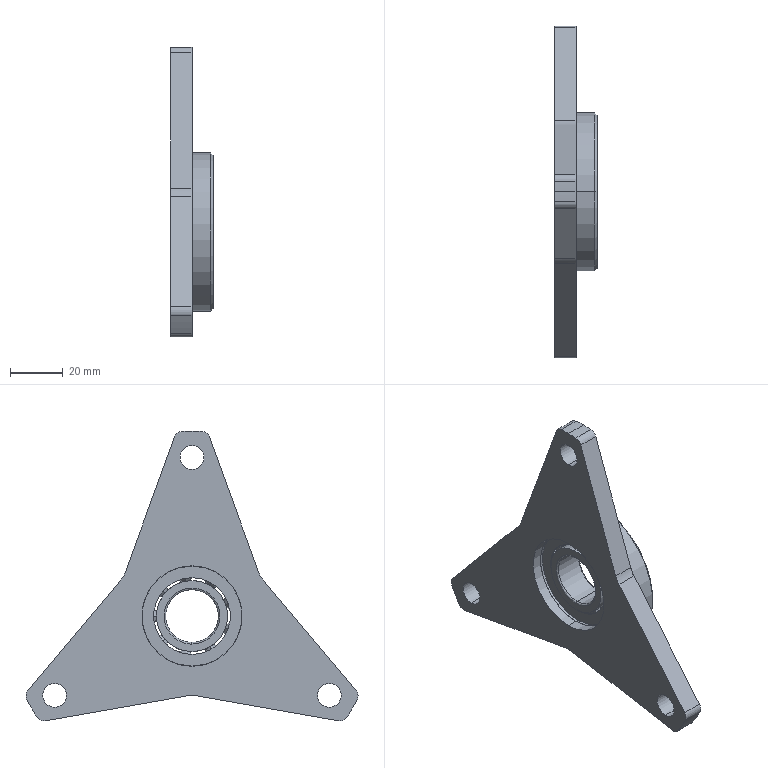Part | SolidWorks | 2 solids | 201 faces | box 16 x 125.605 x 109.685 mm | volume 58698 mm3 | spline 110 | cylinder 49 | plane 38 | cone 4 | commonest cylinder face diameters 37.8 x8 6 x6 9 x6 20 x5 26.9 x4 28.995 x4